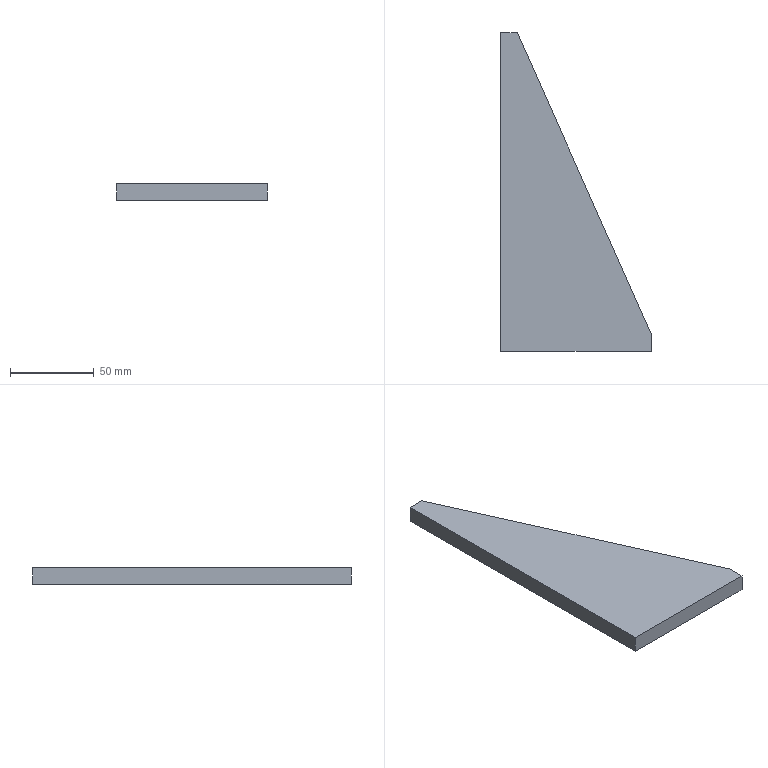Part | SolidWorks | features Extrusion 1 | 1 solid | 7 faces | box 90 x 190 x 10 mm | volume 99000 mm3 | plane 7
STEP:
#1=CARTESIAN_POINT('',(0.,190.,0.));
#2=VERTEX_POINT('',#1);
#3=CARTESIAN_POINT('',(0.,0.,0.));
#4=VERTEX_POINT('',#3);
#5=CARTESIAN_POINT('',(0.,190.,0.));
#6=DIRECTION('',(0.,-1.,0.));
#7=VECTOR('',#6,1000.);
#8=LINE('',#5,#7);
#9=EDGE_CURVE('',#2,#4,#8,.T.);
#10=ORIENTED_EDGE('',*,*,#9,.T.);
#11=CARTESIAN_POINT('',(0.,0.,10.));
#12=VERTEX_POINT('',#11);
#13=CARTESIAN_POINT('',(0.,0.,10.));
#14=DIRECTION('',(0.,0.,-1.));
#15=VECTOR('',#14,1000.);
#16=LINE('',#13,#15);
#17=EDGE_CURVE('',#12,#4,#16,.T.);
#18=ORIENTED_EDGE('',*,*,#17,.F.);
#19=CARTESIAN_POINT('',(0.,190.,10.));
#20=VERTEX_POINT('',#19);
#21=CARTESIAN_POINT('',(0.,190.,10.));
#22=DIRECTION('',(0.,-1.,0.));
#23=VECTOR('',#22,1000.);
#24=LINE('',#21,#23);
#25=EDGE_CURVE('',#20,#12,#24,.T.);
#26=ORIENTED_EDGE('',*,*,#25,.F.);
#27=CARTESIAN_POINT('',(0.,190.,10.));
#28=DIRECTION('',(0.,0.,-1.));
#29=VECTOR('',#28,1000.);
#30=LINE('',#27,#29);
#31=EDGE_CURVE('',#20,#2,#30,.T.);
#32=ORIENTED_EDGE('',*,*,#31,.T.);
#33=EDGE_LOOP('',(#10,#18,#26,#32));
#34=FACE_OUTER_BOUND('',#33,.T.);
#35=CARTESIAN_POINT('',(0.,190.,10.));
#36=DIRECTION('',(1.,0.,0.));
#37=DIRECTION('',(0.,0.,-1.));
#38=AXIS2_PLACEMENT_3D('',#35,#36,#37);
#39=PLANE('',#38);
#40=ADVANCED_FACE('',(#34),#39,.F.);
#41=CARTESIAN_POINT('',(90.,0.,0.));
#42=VERTEX_POINT('',#41);
#43=CARTESIAN_POINT('',(0.,0.,0.));
#44=DIRECTION('',(1.,0.,0.));
#45=VECTOR('',#44,1000.);
#46=LINE('',#43,#45);
#47=EDGE_CURVE('',#4,#42,#46,.T.);
#48=ORIENTED_EDGE('',*,*,#47,.T.);
#49=CARTESIAN_POINT('',(90.,0.,10.));
#50=VERTEX_POINT('',#49);
#51=CARTESIAN_POINT('',(90.,0.,10.));
#52=DIRECTION('',(0.,0.,-1.));
#53=VECTOR('',#52,1000.);
#54=LINE('',#51,#53);
#55=EDGE_CURVE('',#50,#42,#54,.T.);
#56=ORIENTED_EDGE('',*,*,#55,.F.);
#57=CARTESIAN_POINT('',(0.,0.,10.));
#58=DIRECTION('',(1.,0.,0.));
#59=VECTOR('',#58,1000.);
#60=LINE('',#57,#59);
#61=EDGE_CURVE('',#12,#50,#60,.T.);
#62=ORIENTED_EDGE('',*,*,#61,.F.);
#63=ORIENTED_EDGE('',*,*,#17,.T.);
#64=EDGE_LOOP('',(#48,#56,#62,#63));
#65=FACE_OUTER_BOUND('',#64,.T.);
#66=CARTESIAN_POINT('',(0.,0.,10.));
#67=DIRECTION('',(0.,1.,0.));
#68=DIRECTION('',(0.,0.,1.));
#69=AXIS2_PLACEMENT_3D('',#66,#67,#68);
#70=PLANE('',#69);
#71=ADVANCED_FACE('',(#65),#70,.F.);
#72=CARTESIAN_POINT('',(90.,10.,0.));
#73=VERTEX_POINT('',#72);
#74=CARTESIAN_POINT('',(90.,0.,0.));
#75=DIRECTION('',(0.,1.,0.));
#76=VECTOR('',#75,1000.);
#77=LINE('',#74,#76);
#78=EDGE_CURVE('',#42,#73,#77,.T.);
#79=ORIENTED_EDGE('',*,*,#78,.T.);
#80=CARTESIAN_POINT('',(90.,10.,10.));
#81=VERTEX_POINT('',#80);
#82=CARTESIAN_POINT('',(90.,10.,10.));
#83=DIRECTION('',(0.,0.,-1.));
#84=VECTOR('',#83,1000.);
#85=LINE('',#82,#84);
#86=EDGE_CURVE('',#81,#73,#85,.T.);
#87=ORIENTED_EDGE('',*,*,#86,.F.);
#88=CARTESIAN_POINT('',(90.,0.,10.));
#89=DIRECTION('',(0.,1.,0.));
#90=VECTOR('',#89,1000.);
#91=LINE('',#88,#90);
#92=EDGE_CURVE('',#50,#81,#91,.T.);
#93=ORIENTED_EDGE('',*,*,#92,.F.);
#94=ORIENTED_EDGE('',*,*,#55,.T.);
#95=EDGE_LOOP('',(#79,#87,#93,#94));
#96=FACE_OUTER_BOUND('',#95,.T.);
#97=CARTESIAN_POINT('',(90.,0.,10.));
#98=DIRECTION('',(-1.,0.,0.));
#99=DIRECTION('',(0.,0.,1.));
#100=AXIS2_PLACEMENT_3D('',#97,#98,#99);
#101=PLANE('',#100);
#102=ADVANCED_FACE('',(#96),#101,.F.);
#103=CARTESIAN_POINT('',(10.,190.,0.));
#104=VERTEX_POINT('',#103);
#105=CARTESIAN_POINT('',(90.,10.,0.));
#106=DIRECTION('',(-0.4061,0.9138,0.));
#107=VECTOR('',#106,1000.);
#108=LINE('',#105,#107);
#109=EDGE_CURVE('',#73,#104,#108,.T.);
#110=ORIENTED_EDGE('',*,*,#109,.T.);
#111=CARTESIAN_POINT('',(10.,190.,10.));
#112=VERTEX_POINT('',#111);
#113=CARTESIAN_POINT('',(10.,190.,10.));
#114=DIRECTION('',(0.,0.,-1.));
#115=VECTOR('',#114,1000.);
#116=LINE('',#113,#115);
#117=EDGE_CURVE('',#112,#104,#116,.T.);
#118=ORIENTED_EDGE('',*,*,#117,.F.);
#119=CARTESIAN_POINT('',(90.,10.,10.));
#120=DIRECTION('',(-0.4061,0.9138,0.));
#121=VECTOR('',#120,1000.);
#122=LINE('',#119,#121);
#123=EDGE_CURVE('',#81,#112,#122,.T.);
#124=ORIENTED_EDGE('',*,*,#123,.F.);
#125=ORIENTED_EDGE('',*,*,#86,.T.);
#126=EDGE_LOOP('',(#110,#118,#124,#125));
#127=FACE_OUTER_BOUND('',#126,.T.);
#128=CARTESIAN_POINT('',(90.,10.,10.));
#129=DIRECTION('',(-0.9138,-0.4061,0.));
#130=DIRECTION('',(0.4061,-0.9138,0.));
#131=AXIS2_PLACEMENT_3D('',#128,#129,#130);
#132=PLANE('',#131);
#133=ADVANCED_FACE('',(#127),#132,.F.);
#134=CARTESIAN_POINT('',(10.,190.,0.));
#135=DIRECTION('',(-1.,0.,0.));
#136=VECTOR('',#135,1000.);
#137=LINE('',#134,#136);
#138=EDGE_CURVE('',#104,#2,#137,.T.);
#139=ORIENTED_EDGE('',*,*,#138,.T.);
#140=ORIENTED_EDGE('',*,*,#31,.F.);
#141=CARTESIAN_POINT('',(10.,190.,10.));
#142=DIRECTION('',(-1.,0.,0.));
#143=VECTOR('',#142,1000.);
#144=LINE('',#141,#143);
#145=EDGE_CURVE('',#112,#20,#144,.T.);
#146=ORIENTED_EDGE('',*,*,#145,.F.);
#147=ORIENTED_EDGE('',*,*,#117,.T.);
#148=EDGE_LOOP('',(#139,#140,#146,#147));
#149=FACE_OUTER_BOUND('',#148,.T.);
#150=CARTESIAN_POINT('',(10.,190.,10.));
#151=DIRECTION('',(0.,-1.,0.));
#152=DIRECTION('',(1.,0.,0.));
#153=AXIS2_PLACEMENT_3D('',#150,#151,#152);
#154=PLANE('',#153);
#155=ADVANCED_FACE('',(#149),#154,.F.);
#156=ORIENTED_EDGE('',*,*,#25,.T.);
#157=ORIENTED_EDGE('',*,*,#61,.T.);
#158=ORIENTED_EDGE('',*,*,#92,.T.);
#159=ORIENTED_EDGE('',*,*,#123,.T.);
#160=ORIENTED_EDGE('',*,*,#145,.T.);
#161=EDGE_LOOP('',(#156,#157,#158,#159,#160));
#162=FACE_OUTER_BOUND('',#161,.T.);
#163=CARTESIAN_POINT('',(0.,0.,10.));
#164=DIRECTION('',(0.,0.,1.));
#165=DIRECTION('',(1.,0.,0.));
#166=AXIS2_PLACEMENT_3D('',#163,#164,#165);
#167=PLANE('',#166);
#168=ADVANCED_FACE('',(#162),#167,.T.);
#169=ORIENTED_EDGE('',*,*,#9,.F.);
#170=ORIENTED_EDGE('',*,*,#138,.F.);
#171=ORIENTED_EDGE('',*,*,#109,.F.);
#172=ORIENTED_EDGE('',*,*,#78,.F.);
#173=ORIENTED_EDGE('',*,*,#47,.F.);
#174=EDGE_LOOP('',(#169,#170,#171,#172,#173));
#175=FACE_OUTER_BOUND('',#174,.T.);
#176=CARTESIAN_POINT('',(0.,0.,0.));
#177=DIRECTION('',(0.,0.,1.));
#178=DIRECTION('',(1.,0.,0.));
#179=AXIS2_PLACEMENT_3D('',#176,#177,#178);
#180=PLANE('',#179);
#181=ADVANCED_FACE('',(#175),#180,.F.);
#182=CLOSED_SHELL('',(#40,#71,#102,#133,#155,#168,#181));
#183=MANIFOLD_SOLID_BREP('',#182);
#184=CARTESIAN_POINT('',(0.,0.,0.));
#185=DIRECTION('',(0.,0.,1.));
#186=DIRECTION('',(1.,0.,0.));
#187=AXIS2_PLACEMENT_3D('',#184,#185,#186);
#188=(LENGTH_UNIT()NAMED_UNIT(*)SI_UNIT(.MILLI.,.METRE.));
#189=UNCERTAINTY_MEASURE_WITH_UNIT(LENGTH_MEASURE(0.00001),#188,'','');
#190=(NAMED_UNIT(*)PLANE_ANGLE_UNIT()SI_UNIT($,.RADIAN.));
#191=(NAMED_UNIT(*)SI_UNIT($,.STERADIAN.)SOLID_ANGLE_UNIT());
#192=(GEOMETRIC_REPRESENTATION_CONTEXT(3)GLOBAL_UNCERTAINTY_ASSIGNED_CONTEXT((#189))GLOBAL_UNIT_ASSIGNED_CONTEXT((#188,#190,#191))REPRESENTATION_CONTEXT('',''));
#193=ADVANCED_BREP_SHAPE_REPRESENTATION('',(#183,#187),#192);